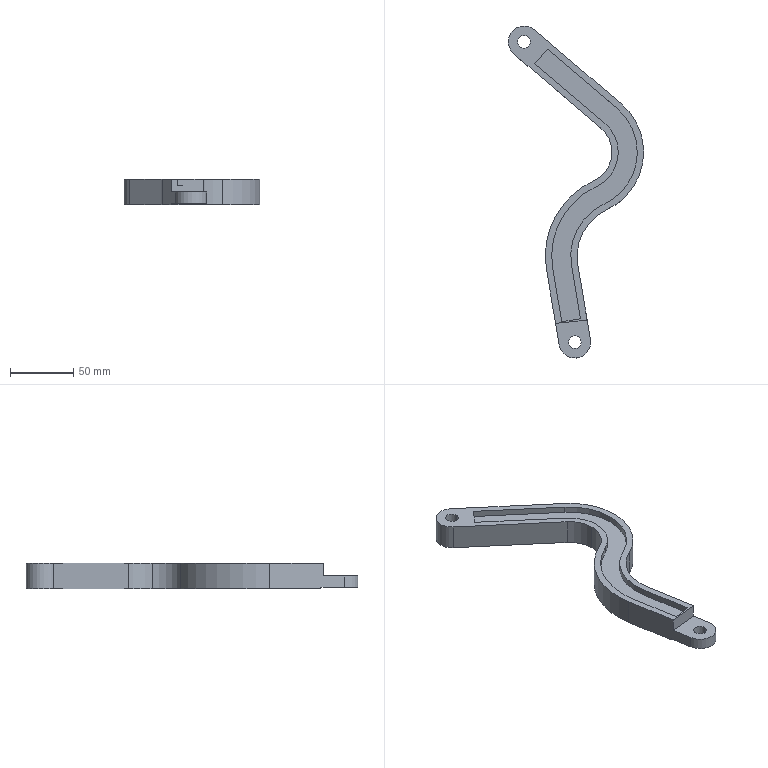Part | SolidWorks | features ICE 3, Cut 1, Extrusion 1 | 1 solid | 50 faces | box 106.703 x 261.653 x 20 mm | volume 108467 mm3 | cylinder 25 | plane 25 | commonest cylinder face diameters 10 x4 60 x4 90 x4 25 x3 50 x2 90.105 x2